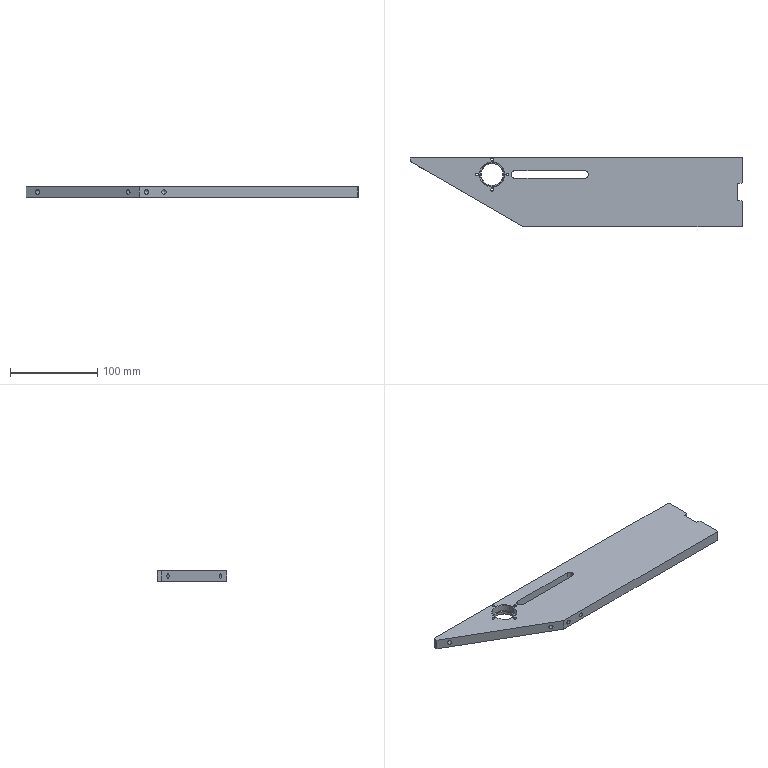CAM job | NX | 3-axis milling, drilling | part box 380 x 80 x 12 mm | stock box 384 x 80 x 12 mm
Tools:
number,name,description,diameter,corner_radius,flute_length,length,flutes
6,D8A45,Milling Tool-5 Parameters,8.0,0.0,50.0,75.0,2
12,3.3ZT,Drilling Tool,3.3,0.0,35.0,50.0,2
4,D10,Milling Tool-5 Parameters,10.0,0.0,50.0,75.0,2
2,D6,Milling Tool-5 Parameters,6.0,0.0,50.0,75.0,2
Operations:
program,operation,operation_type,tool,method,geometry_group,spindle_rpm,surface_speed,feed_per_tooth,feed_cut,feed_plunge,cut_length_mm,path_length_mm,cut_time_min,machine_time_min
1,DRILLING,Operation,D8A45,METHOD,A,3500.0,65.0,0.0357,250.0,0.0,23.75,204.87,0.095,0.1131
1,DRILLING_COPY,Operation,3.3ZT,METHOD,A,1500.0,15.0,0.05,150.0,0.0,69.966,283.721,0.4664,0.4878
1,ZLEVEL_PROFILE,ZLevelMilling,D10,METHOD,A,7000.0,219.0,0.2143,3000.0,1000.0,3406.909,3840.739,1.178,1.221
1,ZLEVEL_PROFILE_COPY,ZLevelMilling,D10,METHOD,A,7000.0,219.0,0.0714,1000.0,1000.0,262.88,689.857,0.2629,0.3056
1,HOLE_MILLING,CylinderMilling,D10,METHOD,A,7000.0,0.0,0.0,2000.0,100.0,839.033,915.033,0.4195,0.4271
1,HOLE_MILLING_COPY,CylinderMilling,D10,METHOD,A,7000.0,0.0,0.0893,1250.0,100.0,424.258,508.258,0.3394,0.3478
1,ZLEVEL_PROFILE_1,ZLevelMilling,D6,METHOD,A,7000.0,131.0,0.1036,1450.0,1000.0,4096.956,4165.956,2.837,2.844
1,PLANAR_MILL,PlanarMilling,D8A45,METHOD,A,7000.0,1495.0,0.0893,1250.0,100.0,311.711,799.981,0.2494,0.2982
1,PLANAR_MILL_COPY,PlanarMilling,D8A45,METHOD,A,7000.0,1495.0,0.0893,1250.0,100.0,261.353,631.709,0.2091,0.2461
1,刀补4,CylinderMilling,D10,METHOD,A,7000.0,0.0,0.0714,1000.0,100.0,238.315,305.815,0.2383,0.2451